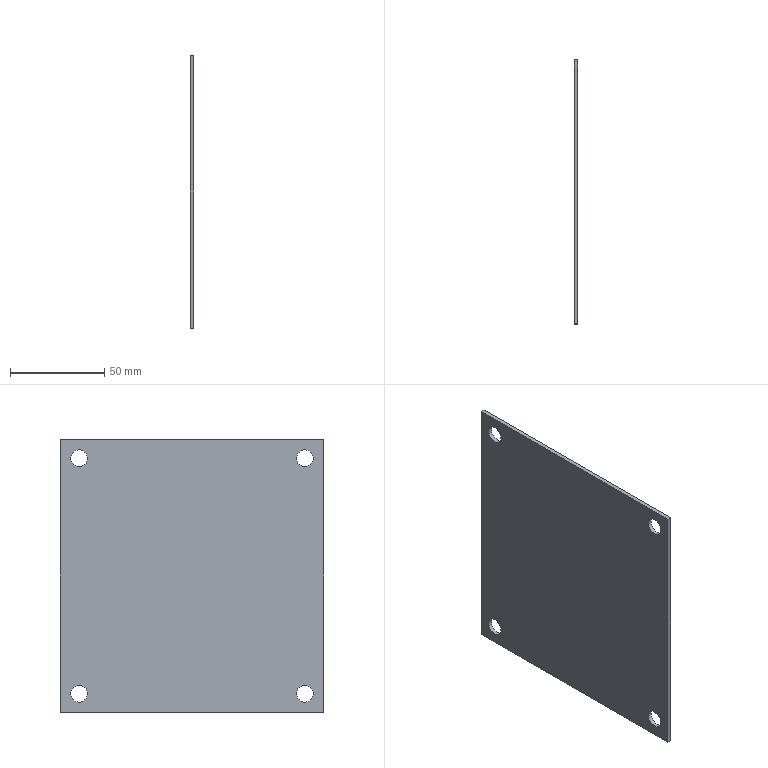Part | NX | features MAIN_BODY 2 | 1 solid | 10 faces | box 2 x 140 x 145 mm | volume 40091 mm3 | plane 6 | cylinder 4 | commonest cylinder face diameters 9 x4
STEP:
#1=CARTESIAN_POINT('',(-1379.5,-376.5,382.));
#2=VERTEX_POINT('',#1);
#3=CARTESIAN_POINT('',(-1379.5,-376.5,386.5));
#4=DIRECTION('',(-1.,0.,0.));
#5=DIRECTION('',(0.,0.,-1.));
#6=AXIS2_PLACEMENT_3D('',#3,#4,#5);
#7=CIRCLE('',#6,4.5);
#8=EDGE_CURVE('',#2,#2,#7,.F.);
#9=ORIENTED_EDGE('',*,*,#8,.F.);
#10=EDGE_LOOP('',(#9));
#11=FACE_BOUND('',#10,.T.);
#12=CARTESIAN_POINT('',(-1379.5,-496.5,382.));
#13=VERTEX_POINT('',#12);
#14=CARTESIAN_POINT('',(-1379.5,-496.5,386.5));
#15=DIRECTION('',(-1.,0.,0.));
#16=DIRECTION('',(0.,0.,-1.));
#17=AXIS2_PLACEMENT_3D('',#14,#15,#16);
#18=CIRCLE('',#17,4.5);
#19=EDGE_CURVE('',#13,#13,#18,.F.);
#20=ORIENTED_EDGE('',*,*,#19,.F.);
#21=EDGE_LOOP('',(#20));
#22=FACE_BOUND('',#21,.T.);
#23=CARTESIAN_POINT('',(-1379.5,-376.5,257.));
#24=VERTEX_POINT('',#23);
#25=CARTESIAN_POINT('',(-1379.5,-376.5,261.5));
#26=DIRECTION('',(-1.,0.,0.));
#27=DIRECTION('',(0.,0.,-1.));
#28=AXIS2_PLACEMENT_3D('',#25,#26,#27);
#29=CIRCLE('',#28,4.5);
#30=EDGE_CURVE('',#24,#24,#29,.F.);
#31=ORIENTED_EDGE('',*,*,#30,.F.);
#32=EDGE_LOOP('',(#31));
#33=FACE_BOUND('',#32,.T.);
#34=CARTESIAN_POINT('',(-1379.5,-496.5,257.));
#35=VERTEX_POINT('',#34);
#36=CARTESIAN_POINT('',(-1379.5,-496.5,261.5));
#37=DIRECTION('',(-1.,0.,0.));
#38=DIRECTION('',(0.,0.,-1.));
#39=AXIS2_PLACEMENT_3D('',#36,#37,#38);
#40=CIRCLE('',#39,4.5);
#41=EDGE_CURVE('',#35,#35,#40,.F.);
#42=ORIENTED_EDGE('',*,*,#41,.F.);
#43=EDGE_LOOP('',(#42));
#44=FACE_BOUND('',#43,.T.);
#45=CARTESIAN_POINT('',(-1379.5,-366.5,251.5));
#46=VERTEX_POINT('',#45);
#47=CARTESIAN_POINT('',(-1379.5,-506.5,251.5));
#48=VERTEX_POINT('',#47);
#49=CARTESIAN_POINT('',(-1379.5,-366.5,251.5));
#50=DIRECTION('',(0.,-1.,0.));
#51=VECTOR('',#50,1000.);
#52=LINE('',#49,#51);
#53=EDGE_CURVE('',#46,#48,#52,.T.);
#54=ORIENTED_EDGE('',*,*,#53,.F.);
#55=CARTESIAN_POINT('',(-1379.5,-366.5,396.5));
#56=VERTEX_POINT('',#55);
#57=CARTESIAN_POINT('',(-1379.5,-366.5,396.5));
#58=DIRECTION('',(0.,0.,1.));
#59=VECTOR('',#58,1000.);
#60=LINE('',#57,#59);
#61=EDGE_CURVE('',#56,#46,#60,.F.);
#62=ORIENTED_EDGE('',*,*,#61,.F.);
#63=CARTESIAN_POINT('',(-1379.5,-506.5,396.5));
#64=VERTEX_POINT('',#63);
#65=CARTESIAN_POINT('',(-1379.5,-366.5,396.5));
#66=DIRECTION('',(0.,1.,0.));
#67=VECTOR('',#66,1000.);
#68=LINE('',#65,#67);
#69=EDGE_CURVE('',#56,#64,#68,.F.);
#70=ORIENTED_EDGE('',*,*,#69,.T.);
#71=CARTESIAN_POINT('',(-1379.5,-506.5,396.5));
#72=DIRECTION('',(0.,0.,1.));
#73=VECTOR('',#72,1000.);
#74=LINE('',#71,#73);
#75=EDGE_CURVE('',#64,#48,#74,.F.);
#76=ORIENTED_EDGE('',*,*,#75,.T.);
#77=EDGE_LOOP('',(#54,#62,#70,#76));
#78=FACE_BOUND('',#77,.T.);
#79=CARTESIAN_POINT('',(-1379.5,-366.5,396.5));
#80=DIRECTION('',(1.,0.,0.));
#81=DIRECTION('',(0.,0.,-1.));
#82=AXIS2_PLACEMENT_3D('',#79,#80,#81);
#83=PLANE('',#82);
#84=ADVANCED_FACE('',(#11,#22,#33,#44,#78),#83,.T.);
#85=ORIENTED_EDGE('',*,*,#69,.F.);
#86=CARTESIAN_POINT('',(-1381.5,-366.5,396.5));
#87=VERTEX_POINT('',#86);
#88=CARTESIAN_POINT('',(-1375.5,-366.5,396.5));
#89=DIRECTION('',(-1.,0.,0.));
#90=VECTOR('',#89,1000.);
#91=LINE('',#88,#90);
#92=EDGE_CURVE('',#56,#87,#91,.T.);
#93=ORIENTED_EDGE('',*,*,#92,.T.);
#94=CARTESIAN_POINT('',(-1381.5,-506.5,396.5));
#95=VERTEX_POINT('',#94);
#96=CARTESIAN_POINT('',(-1381.5,-366.5,396.5));
#97=DIRECTION('',(0.,1.,0.));
#98=VECTOR('',#97,1000.);
#99=LINE('',#96,#98);
#100=EDGE_CURVE('',#87,#95,#99,.F.);
#101=ORIENTED_EDGE('',*,*,#100,.T.);
#102=CARTESIAN_POINT('',(-1375.5,-506.5,396.5));
#103=DIRECTION('',(1.,0.,0.));
#104=VECTOR('',#103,1000.);
#105=LINE('',#102,#104);
#106=EDGE_CURVE('',#64,#95,#105,.F.);
#107=ORIENTED_EDGE('',*,*,#106,.F.);
#108=EDGE_LOOP('',(#85,#93,#101,#107));
#109=FACE_BOUND('',#108,.T.);
#110=CARTESIAN_POINT('',(-1375.5,-366.5,396.5));
#111=DIRECTION('',(0.,0.,-1.));
#112=DIRECTION('',(-1.,0.,0.));
#113=AXIS2_PLACEMENT_3D('',#110,#111,#112);
#114=PLANE('',#113);
#115=ADVANCED_FACE('',(#109),#114,.F.);
#116=CARTESIAN_POINT('',(-1381.5,-376.5,382.));
#117=VERTEX_POINT('',#116);
#118=CARTESIAN_POINT('',(-1381.5,-376.5,386.5));
#119=DIRECTION('',(-1.,0.,0.));
#120=DIRECTION('',(0.,0.,-1.));
#121=AXIS2_PLACEMENT_3D('',#118,#119,#120);
#122=CIRCLE('',#121,4.5);
#123=EDGE_CURVE('',#117,#117,#122,.T.);
#124=ORIENTED_EDGE('',*,*,#123,.F.);
#125=EDGE_LOOP('',(#124));
#126=FACE_BOUND('',#125,.T.);
#127=CARTESIAN_POINT('',(-1381.5,-496.5,382.));
#128=VERTEX_POINT('',#127);
#129=CARTESIAN_POINT('',(-1381.5,-496.5,386.5));
#130=DIRECTION('',(-1.,0.,0.));
#131=DIRECTION('',(0.,0.,-1.));
#132=AXIS2_PLACEMENT_3D('',#129,#130,#131);
#133=CIRCLE('',#132,4.5);
#134=EDGE_CURVE('',#128,#128,#133,.T.);
#135=ORIENTED_EDGE('',*,*,#134,.F.);
#136=EDGE_LOOP('',(#135));
#137=FACE_BOUND('',#136,.T.);
#138=CARTESIAN_POINT('',(-1381.5,-376.5,257.));
#139=VERTEX_POINT('',#138);
#140=CARTESIAN_POINT('',(-1381.5,-376.5,261.5));
#141=DIRECTION('',(-1.,0.,0.));
#142=DIRECTION('',(0.,0.,-1.));
#143=AXIS2_PLACEMENT_3D('',#140,#141,#142);
#144=CIRCLE('',#143,4.5);
#145=EDGE_CURVE('',#139,#139,#144,.T.);
#146=ORIENTED_EDGE('',*,*,#145,.F.);
#147=EDGE_LOOP('',(#146));
#148=FACE_BOUND('',#147,.T.);
#149=CARTESIAN_POINT('',(-1381.5,-496.5,257.));
#150=VERTEX_POINT('',#149);
#151=CARTESIAN_POINT('',(-1381.5,-496.5,261.5));
#152=DIRECTION('',(-1.,0.,0.));
#153=DIRECTION('',(0.,0.,-1.));
#154=AXIS2_PLACEMENT_3D('',#151,#152,#153);
#155=CIRCLE('',#154,4.5);
#156=EDGE_CURVE('',#150,#150,#155,.T.);
#157=ORIENTED_EDGE('',*,*,#156,.F.);
#158=EDGE_LOOP('',(#157));
#159=FACE_BOUND('',#158,.T.);
#160=ORIENTED_EDGE('',*,*,#100,.F.);
#161=CARTESIAN_POINT('',(-1381.5,-366.5,251.5));
#162=VERTEX_POINT('',#161);
#163=CARTESIAN_POINT('',(-1381.5,-366.5,396.5));
#164=DIRECTION('',(0.,0.,-1.));
#165=VECTOR('',#164,1000.);
#166=LINE('',#163,#165);
#167=EDGE_CURVE('',#87,#162,#166,.T.);
#168=ORIENTED_EDGE('',*,*,#167,.T.);
#169=CARTESIAN_POINT('',(-1381.5,-506.5,251.5));
#170=VERTEX_POINT('',#169);
#171=CARTESIAN_POINT('',(-1381.5,-366.5,251.5));
#172=DIRECTION('',(0.,1.,0.));
#173=VECTOR('',#172,1000.);
#174=LINE('',#171,#173);
#175=EDGE_CURVE('',#162,#170,#174,.F.);
#176=ORIENTED_EDGE('',*,*,#175,.T.);
#177=CARTESIAN_POINT('',(-1381.5,-506.5,396.5));
#178=DIRECTION('',(0.,0.,1.));
#179=VECTOR('',#178,1000.);
#180=LINE('',#177,#179);
#181=EDGE_CURVE('',#95,#170,#180,.F.);
#182=ORIENTED_EDGE('',*,*,#181,.F.);
#183=EDGE_LOOP('',(#160,#168,#176,#182));
#184=FACE_BOUND('',#183,.T.);
#185=CARTESIAN_POINT('',(-1381.5,-366.5,396.5));
#186=DIRECTION('',(1.,0.,0.));
#187=DIRECTION('',(0.,0.,-1.));
#188=AXIS2_PLACEMENT_3D('',#185,#186,#187);
#189=PLANE('',#188);
#190=ADVANCED_FACE('',(#126,#137,#148,#159,#184),#189,.F.);
#191=CARTESIAN_POINT('',(-1375.5,-366.5,251.5));
#192=DIRECTION('',(-1.,0.,0.));
#193=VECTOR('',#192,1000.);
#194=LINE('',#191,#193);
#195=EDGE_CURVE('',#46,#162,#194,.T.);
#196=ORIENTED_EDGE('',*,*,#195,.F.);
#197=ORIENTED_EDGE('',*,*,#53,.T.);
#198=CARTESIAN_POINT('',(-1375.5,-506.5,251.5));
#199=DIRECTION('',(1.,0.,0.));
#200=VECTOR('',#199,1000.);
#201=LINE('',#198,#200);
#202=EDGE_CURVE('',#48,#170,#201,.F.);
#203=ORIENTED_EDGE('',*,*,#202,.T.);
#204=ORIENTED_EDGE('',*,*,#175,.F.);
#205=EDGE_LOOP('',(#196,#197,#203,#204));
#206=FACE_BOUND('',#205,.T.);
#207=CARTESIAN_POINT('',(-1375.5,-366.5,251.5));
#208=DIRECTION('',(0.,0.,-1.));
#209=DIRECTION('',(-1.,0.,0.));
#210=AXIS2_PLACEMENT_3D('',#207,#208,#209);
#211=PLANE('',#210);
#212=ADVANCED_FACE('',(#206),#211,.T.);
#213=ORIENTED_EDGE('',*,*,#181,.T.);
#214=ORIENTED_EDGE('',*,*,#202,.F.);
#215=ORIENTED_EDGE('',*,*,#75,.F.);
#216=ORIENTED_EDGE('',*,*,#106,.T.);
#217=EDGE_LOOP('',(#213,#214,#215,#216));
#218=FACE_BOUND('',#217,.T.);
#219=CARTESIAN_POINT('',(-1375.5,-506.5,396.5));
#220=DIRECTION('',(0.,-1.,0.));
#221=DIRECTION('',(0.,0.,1.));
#222=AXIS2_PLACEMENT_3D('',#219,#220,#221);
#223=PLANE('',#222);
#224=ADVANCED_FACE('',(#218),#223,.T.);
#225=ORIENTED_EDGE('',*,*,#167,.F.);
#226=ORIENTED_EDGE('',*,*,#92,.F.);
#227=ORIENTED_EDGE('',*,*,#61,.T.);
#228=ORIENTED_EDGE('',*,*,#195,.T.);
#229=EDGE_LOOP('',(#225,#226,#227,#228));
#230=FACE_BOUND('',#229,.T.);
#231=CARTESIAN_POINT('',(-1375.5,-366.5,396.5));
#232=DIRECTION('',(0.,-1.,0.));
#233=DIRECTION('',(0.,0.,1.));
#234=AXIS2_PLACEMENT_3D('',#231,#232,#233);
#235=PLANE('',#234);
#236=ADVANCED_FACE('',(#230),#235,.F.);
#237=ORIENTED_EDGE('',*,*,#41,.T.);
#238=EDGE_LOOP('',(#237));
#239=FACE_BOUND('',#238,.T.);
#240=ORIENTED_EDGE('',*,*,#156,.T.);
#241=EDGE_LOOP('',(#240));
#242=FACE_BOUND('',#241,.T.);
#243=CARTESIAN_POINT('',(-1375.5,-496.5,261.5));
#244=DIRECTION('',(-1.,0.,0.));
#245=DIRECTION('',(0.,0.,1.));
#246=AXIS2_PLACEMENT_3D('',#243,#244,#245);
#247=CYLINDRICAL_SURFACE('',#246,4.5);
#248=ADVANCED_FACE('',(#239,#242),#247,.F.);
#249=ORIENTED_EDGE('',*,*,#30,.T.);
#250=EDGE_LOOP('',(#249));
#251=FACE_BOUND('',#250,.T.);
#252=ORIENTED_EDGE('',*,*,#145,.T.);
#253=EDGE_LOOP('',(#252));
#254=FACE_BOUND('',#253,.T.);
#255=CARTESIAN_POINT('',(-1375.5,-376.5,261.5));
#256=DIRECTION('',(-1.,0.,0.));
#257=DIRECTION('',(0.,0.,1.));
#258=AXIS2_PLACEMENT_3D('',#255,#256,#257);
#259=CYLINDRICAL_SURFACE('',#258,4.5);
#260=ADVANCED_FACE('',(#251,#254),#259,.F.);
#261=ORIENTED_EDGE('',*,*,#19,.T.);
#262=EDGE_LOOP('',(#261));
#263=FACE_BOUND('',#262,.T.);
#264=ORIENTED_EDGE('',*,*,#134,.T.);
#265=EDGE_LOOP('',(#264));
#266=FACE_BOUND('',#265,.T.);
#267=CARTESIAN_POINT('',(-1375.5,-496.5,386.5));
#268=DIRECTION('',(-1.,0.,0.));
#269=DIRECTION('',(0.,0.,1.));
#270=AXIS2_PLACEMENT_3D('',#267,#268,#269);
#271=CYLINDRICAL_SURFACE('',#270,4.5);
#272=ADVANCED_FACE('',(#263,#266),#271,.F.);
#273=ORIENTED_EDGE('',*,*,#8,.T.);
#274=EDGE_LOOP('',(#273));
#275=FACE_BOUND('',#274,.T.);
#276=ORIENTED_EDGE('',*,*,#123,.T.);
#277=EDGE_LOOP('',(#276));
#278=FACE_BOUND('',#277,.T.);
#279=CARTESIAN_POINT('',(-1375.5,-376.5,386.5));
#280=DIRECTION('',(-1.,0.,0.));
#281=DIRECTION('',(0.,0.,1.));
#282=AXIS2_PLACEMENT_3D('',#279,#280,#281);
#283=CYLINDRICAL_SURFACE('',#282,4.5);
#284=ADVANCED_FACE('',(#275,#278),#283,.F.);
#285=CLOSED_SHELL('',(#84,#115,#190,#212,#224,#236,#248,#260,#272,#284));
#286=MANIFOLD_SOLID_BREP('',#285);
#287=(LENGTH_UNIT()NAMED_UNIT(*)SI_UNIT(.MILLI.,.METRE.));
#288=UNCERTAINTY_MEASURE_WITH_UNIT(LENGTH_MEASURE(0.00001),#287,'','');
#289=(NAMED_UNIT(*)PLANE_ANGLE_UNIT()SI_UNIT($,.RADIAN.));
#290=(NAMED_UNIT(*)SI_UNIT($,.STERADIAN.)SOLID_ANGLE_UNIT());
#291=(GEOMETRIC_REPRESENTATION_CONTEXT(3)GLOBAL_UNCERTAINTY_ASSIGNED_CONTEXT((#288))GLOBAL_UNIT_ASSIGNED_CONTEXT((#287,#289,#290))REPRESENTATION_CONTEXT('',''));
#292=ADVANCED_BREP_SHAPE_REPRESENTATION('',(#286),#291);